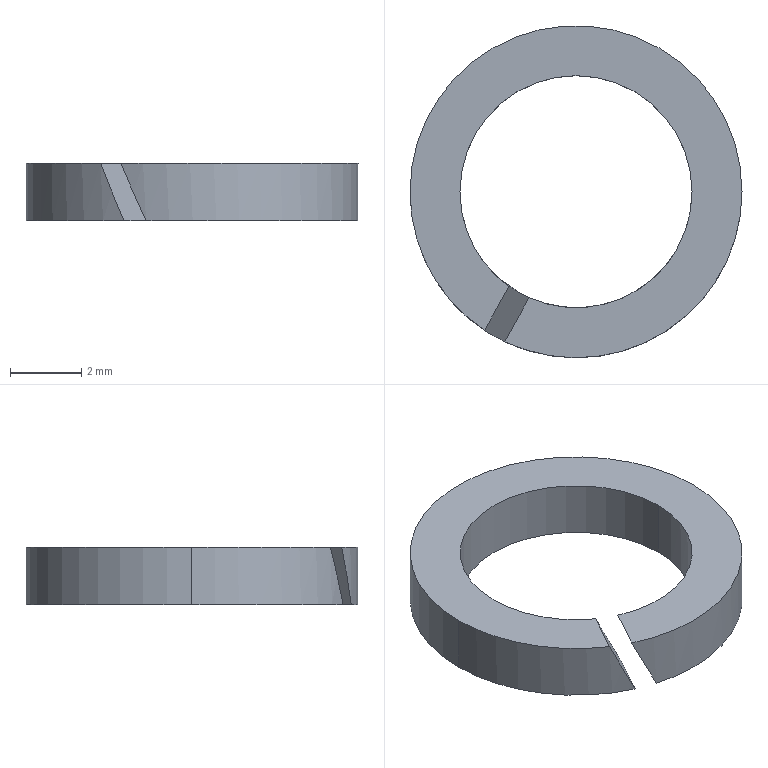Part | SolidWorks | features BaseBody 1 | 1 solid | 10 faces | box 9.3 x 9.3 x 1.6 mm | volume 54.128 mm3 | cylinder 6 | plane 4 | commonest cylinder face diameters 6.5 x3 9.3 x3
STEP:
#1=CARTESIAN_POINT('',(-40.153,-58.725,-65.029));
#2=VERTEX_POINT('',#1);
#3=CARTESIAN_POINT('',(-44.719,-61.697,-65.029));
#4=VERTEX_POINT('',#3);
#5=CARTESIAN_POINT('',(-43.403,-58.725,-65.029));
#6=DIRECTION('',(-0.000001053,0.,-1.));
#7=DIRECTION('',(-1.,0.,0.000001053));
#8=AXIS2_PLACEMENT_3D('',#5,#6,#7);
#9=CIRCLE('',#8,3.25);
#10=EDGE_CURVE('',#2,#4,#9,.T.);
#11=ORIENTED_EDGE('',*,*,#10,.F.);
#12=CARTESIAN_POINT('',(-40.153,-58.725,-66.629));
#13=VERTEX_POINT('',#12);
#14=CARTESIAN_POINT('',(-40.153,-58.725,-65.029));
#15=DIRECTION('',(-0.000001053,0.,-1.));
#16=VECTOR('',#15,1000.);
#17=LINE('',#14,#16);
#18=EDGE_CURVE('',#2,#13,#17,.T.);
#19=ORIENTED_EDGE('',*,*,#18,.T.);
#20=CARTESIAN_POINT('',(-43.991,-61.921,-66.629));
#21=VERTEX_POINT('',#20);
#22=CARTESIAN_POINT('',(-43.403,-58.725,-66.629));
#23=DIRECTION('',(0.000001053,0.,1.));
#24=DIRECTION('',(-1.,0.,0.000001053));
#25=AXIS2_PLACEMENT_3D('',#22,#23,#24);
#26=CIRCLE('',#25,3.25);
#27=EDGE_CURVE('',#21,#13,#26,.T.);
#28=ORIENTED_EDGE('',*,*,#27,.F.);
#29=CARTESIAN_POINT('',(-44.719,-61.697,-65.029));
#30=CARTESIAN_POINT('',(-44.486,-61.8,-65.574));
#31=CARTESIAN_POINT('',(-44.242,-61.875,-66.11));
#32=CARTESIAN_POINT('',(-43.991,-61.921,-66.629));
#33=(BOUNDED_CURVE()B_SPLINE_CURVE(3,(#29,#30,#31,#32),.UNSPECIFIED.,.F.,.T.)B_SPLINE_CURVE_WITH_KNOTS((4,4),(4.8,5.035),.UNSPECIFIED.)CURVE()GEOMETRIC_REPRESENTATION_ITEM()RATIONAL_B_SPLINE_CURVE((1.,0.9954,0.9954,1.))REPRESENTATION_ITEM(''));
#34=EDGE_CURVE('',#4,#21,#33,.T.);
#35=ORIENTED_EDGE('',*,*,#34,.F.);
#36=EDGE_LOOP('',(#11,#19,#28,#35));
#37=FACE_OUTER_BOUND('',#36,.T.);
#38=CARTESIAN_POINT('',(-43.403,-58.725,-65.029));
#39=DIRECTION('',(-0.000001053,0.,-1.));
#40=DIRECTION('',(-1.,0.,0.000001053));
#41=AXIS2_PLACEMENT_3D('',#38,#39,#40);
#42=CYLINDRICAL_SURFACE('',#41,3.25);
#43=ADVANCED_FACE('',(#37),#42,.F.);
#44=ORIENTED_EDGE('',*,*,#18,.F.);
#45=CARTESIAN_POINT('',(-46.653,-58.725,-65.029));
#46=VERTEX_POINT('',#45);
#47=CARTESIAN_POINT('',(-43.403,-58.725,-65.029));
#48=DIRECTION('',(-0.000001053,0.,-1.));
#49=DIRECTION('',(-1.,0.,0.000001053));
#50=AXIS2_PLACEMENT_3D('',#47,#48,#49);
#51=CIRCLE('',#50,3.25);
#52=EDGE_CURVE('',#46,#2,#51,.T.);
#53=ORIENTED_EDGE('',*,*,#52,.F.);
#54=CARTESIAN_POINT('',(-46.653,-58.725,-66.629));
#55=VERTEX_POINT('',#54);
#56=CARTESIAN_POINT('',(-46.653,-58.725,-65.029));
#57=DIRECTION('',(-0.000001053,0.,-1.));
#58=VECTOR('',#57,1000.);
#59=LINE('',#56,#58);
#60=EDGE_CURVE('',#46,#55,#59,.T.);
#61=ORIENTED_EDGE('',*,*,#60,.T.);
#62=CARTESIAN_POINT('',(-43.403,-58.725,-66.629));
#63=DIRECTION('',(0.000001053,0.,1.));
#64=DIRECTION('',(-1.,0.,0.000001053));
#65=AXIS2_PLACEMENT_3D('',#62,#63,#64);
#66=CIRCLE('',#65,3.25);
#67=EDGE_CURVE('',#13,#55,#66,.T.);
#68=ORIENTED_EDGE('',*,*,#67,.F.);
#69=EDGE_LOOP('',(#44,#53,#61,#68));
#70=FACE_OUTER_BOUND('',#69,.T.);
#71=CARTESIAN_POINT('',(-43.403,-58.725,-65.029));
#72=DIRECTION('',(-0.000001053,0.,-1.));
#73=DIRECTION('',(-1.,0.,0.000001053));
#74=AXIS2_PLACEMENT_3D('',#71,#72,#73);
#75=CYLINDRICAL_SURFACE('',#74,3.25);
#76=ADVANCED_FACE('',(#70),#75,.F.);
#77=CARTESIAN_POINT('',(-38.753,-58.725,-65.029));
#78=VERTEX_POINT('',#77);
#79=CARTESIAN_POINT('',(-48.053,-58.725,-65.029));
#80=VERTEX_POINT('',#79);
#81=CARTESIAN_POINT('',(-43.403,-58.725,-65.029));
#82=DIRECTION('',(0.000001053,0.,1.));
#83=DIRECTION('',(-1.,0.,0.000001053));
#84=AXIS2_PLACEMENT_3D('',#81,#82,#83);
#85=CIRCLE('',#84,4.65);
#86=EDGE_CURVE('',#78,#80,#85,.T.);
#87=ORIENTED_EDGE('',*,*,#86,.F.);
#88=CARTESIAN_POINT('',(-38.753,-58.725,-66.629));
#89=VERTEX_POINT('',#88);
#90=CARTESIAN_POINT('',(-38.753,-58.725,-65.029));
#91=DIRECTION('',(-0.000001053,0.,-1.));
#92=VECTOR('',#91,1000.);
#93=LINE('',#90,#92);
#94=EDGE_CURVE('',#78,#89,#93,.T.);
#95=ORIENTED_EDGE('',*,*,#94,.T.);
#96=CARTESIAN_POINT('',(-48.053,-58.725,-66.629));
#97=VERTEX_POINT('',#96);
#98=CARTESIAN_POINT('',(-43.403,-58.725,-66.629));
#99=DIRECTION('',(0.000001053,0.,1.));
#100=DIRECTION('',(-1.,0.,0.000001053));
#101=AXIS2_PLACEMENT_3D('',#98,#99,#100);
#102=CIRCLE('',#101,4.65);
#103=EDGE_CURVE('',#89,#97,#102,.T.);
#104=ORIENTED_EDGE('',*,*,#103,.T.);
#105=CARTESIAN_POINT('',(-48.053,-58.725,-65.029));
#106=DIRECTION('',(-0.000001053,0.,-1.));
#107=VECTOR('',#106,1000.);
#108=LINE('',#105,#107);
#109=EDGE_CURVE('',#80,#97,#108,.T.);
#110=ORIENTED_EDGE('',*,*,#109,.F.);
#111=EDGE_LOOP('',(#87,#95,#104,#110));
#112=FACE_OUTER_BOUND('',#111,.T.);
#113=CARTESIAN_POINT('',(-43.403,-58.725,-65.029));
#114=DIRECTION('',(-0.000001053,0.,-1.));
#115=DIRECTION('',(-1.,0.,0.000001053));
#116=AXIS2_PLACEMENT_3D('',#113,#114,#115);
#117=CYLINDRICAL_SURFACE('',#116,4.65);
#118=ADVANCED_FACE('',(#112),#117,.T.);
#119=CARTESIAN_POINT('',(-45.964,-62.607,-65.029));
#120=VERTEX_POINT('',#119);
#121=CARTESIAN_POINT('',(-43.403,-58.725,-65.029));
#122=DIRECTION('',(0.000001053,0.,1.));
#123=DIRECTION('',(-1.,0.,0.000001053));
#124=AXIS2_PLACEMENT_3D('',#121,#122,#123);
#125=CIRCLE('',#124,4.65);
#126=EDGE_CURVE('',#80,#120,#125,.T.);
#127=ORIENTED_EDGE('',*,*,#126,.F.);
#128=ORIENTED_EDGE('',*,*,#109,.T.);
#129=CARTESIAN_POINT('',(-45.31,-62.966,-66.629));
#130=VERTEX_POINT('',#129);
#131=CARTESIAN_POINT('',(-43.403,-58.725,-66.629));
#132=DIRECTION('',(0.000001053,0.,1.));
#133=DIRECTION('',(-1.,0.,0.000001053));
#134=AXIS2_PLACEMENT_3D('',#131,#132,#133);
#135=CIRCLE('',#134,4.65);
#136=EDGE_CURVE('',#97,#130,#135,.T.);
#137=ORIENTED_EDGE('',*,*,#136,.T.);
#138=CARTESIAN_POINT('',(-45.31,-62.966,-66.629));
#139=CARTESIAN_POINT('',(-45.537,-62.864,-66.096));
#140=CARTESIAN_POINT('',(-45.756,-62.744,-65.562));
#141=CARTESIAN_POINT('',(-45.964,-62.607,-65.029));
#142=(BOUNDED_CURVE()B_SPLINE_CURVE(3,(#138,#139,#140,#141),.UNSPECIFIED.,.F.,.F.)B_SPLINE_CURVE_WITH_KNOTS((4,4),(1.489,1.65),.UNSPECIFIED.)CURVE()GEOMETRIC_REPRESENTATION_ITEM()RATIONAL_B_SPLINE_CURVE((1.,0.9979,0.9979,1.))REPRESENTATION_ITEM(''));
#143=EDGE_CURVE('',#130,#120,#142,.T.);
#144=ORIENTED_EDGE('',*,*,#143,.T.);
#145=EDGE_LOOP('',(#127,#128,#137,#144));
#146=FACE_OUTER_BOUND('',#145,.T.);
#147=CARTESIAN_POINT('',(-43.403,-58.725,-65.029));
#148=DIRECTION('',(-0.000001053,0.,-1.));
#149=DIRECTION('',(-1.,0.,0.000001053));
#150=AXIS2_PLACEMENT_3D('',#147,#148,#149);
#151=CYLINDRICAL_SURFACE('',#150,4.65);
#152=ADVANCED_FACE('',(#146),#151,.T.);
#153=CARTESIAN_POINT('',(-45.284,-61.375,-65.029));
#154=VERTEX_POINT('',#153);
#155=CARTESIAN_POINT('',(-45.627,-61.997,-65.029));
#156=DIRECTION('',(-0.483,-0.8756,0.));
#157=VECTOR('',#156,1000.);
#158=LINE('',#155,#157);
#159=EDGE_CURVE('',#154,#120,#158,.T.);
#160=ORIENTED_EDGE('',*,*,#159,.F.);
#161=CARTESIAN_POINT('',(-43.403,-58.725,-65.029));
#162=DIRECTION('',(-0.000001053,0.,-1.));
#163=DIRECTION('',(-1.,0.,0.000001053));
#164=AXIS2_PLACEMENT_3D('',#161,#162,#163);
#165=CIRCLE('',#164,3.25);
#166=EDGE_CURVE('',#154,#46,#165,.T.);
#167=ORIENTED_EDGE('',*,*,#166,.T.);
#168=ORIENTED_EDGE('',*,*,#52,.T.);
#169=ORIENTED_EDGE('',*,*,#10,.T.);
#170=CARTESIAN_POINT('',(-45.397,-62.926,-65.029));
#171=VERTEX_POINT('',#170);
#172=CARTESIAN_POINT('',(-45.021,-62.243,-65.029));
#173=DIRECTION('',(-0.483,-0.8756,0.));
#174=VECTOR('',#173,1000.);
#175=LINE('',#172,#174);
#176=EDGE_CURVE('',#4,#171,#175,.T.);
#177=ORIENTED_EDGE('',*,*,#176,.T.);
#178=CARTESIAN_POINT('',(-43.403,-58.725,-65.029));
#179=DIRECTION('',(0.000001053,0.,1.));
#180=DIRECTION('',(-1.,0.,0.000001053));
#181=AXIS2_PLACEMENT_3D('',#178,#179,#180);
#182=CIRCLE('',#181,4.65);
#183=EDGE_CURVE('',#171,#78,#182,.T.);
#184=ORIENTED_EDGE('',*,*,#183,.T.);
#185=ORIENTED_EDGE('',*,*,#86,.T.);
#186=ORIENTED_EDGE('',*,*,#126,.T.);
#187=EDGE_LOOP('',(#160,#167,#168,#169,#177,#184,#185,#186));
#188=FACE_OUTER_BOUND('',#187,.T.);
#189=CARTESIAN_POINT('',(-43.403,-58.725,-65.029));
#190=DIRECTION('',(0.000001053,0.,1.));
#191=DIRECTION('',(1.,0.,-0.000001053));
#192=AXIS2_PLACEMENT_3D('',#189,#190,#191);
#193=PLANE('',#192);
#194=ADVANCED_FACE('',(#188),#193,.T.);
#195=ORIENTED_EDGE('',*,*,#60,.F.);
#196=ORIENTED_EDGE('',*,*,#166,.F.);
#197=CARTESIAN_POINT('',(-44.63,-61.735,-66.629));
#198=VERTEX_POINT('',#197);
#199=CARTESIAN_POINT('',(-44.63,-61.735,-66.629));
#200=CARTESIAN_POINT('',(-44.862,-61.64,-66.097));
#201=CARTESIAN_POINT('',(-45.081,-61.52,-65.561));
#202=CARTESIAN_POINT('',(-45.284,-61.375,-65.029));
#203=(BOUNDED_CURVE()B_SPLINE_CURVE(3,(#199,#200,#201,#202),.UNSPECIFIED.,.F.,.F.)B_SPLINE_CURVE_WITH_KNOTS((4,4),(1.454,1.684),.UNSPECIFIED.)CURVE()GEOMETRIC_REPRESENTATION_ITEM()RATIONAL_B_SPLINE_CURVE((1.,0.9956,0.9956,1.))REPRESENTATION_ITEM(''));
#204=EDGE_CURVE('',#198,#154,#203,.T.);
#205=ORIENTED_EDGE('',*,*,#204,.F.);
#206=CARTESIAN_POINT('',(-43.403,-58.725,-66.629));
#207=DIRECTION('',(0.000001053,0.,1.));
#208=DIRECTION('',(-1.,0.,0.000001053));
#209=AXIS2_PLACEMENT_3D('',#206,#207,#208);
#210=CIRCLE('',#209,3.25);
#211=EDGE_CURVE('',#55,#198,#210,.T.);
#212=ORIENTED_EDGE('',*,*,#211,.F.);
#213=EDGE_LOOP('',(#195,#196,#205,#212));
#214=FACE_OUTER_BOUND('',#213,.T.);
#215=CARTESIAN_POINT('',(-43.403,-58.725,-65.029));
#216=DIRECTION('',(-0.000001053,0.,-1.));
#217=DIRECTION('',(-1.,0.,0.000001053));
#218=AXIS2_PLACEMENT_3D('',#215,#216,#217);
#219=CYLINDRICAL_SURFACE('',#218,3.25);
#220=ADVANCED_FACE('',(#214),#219,.F.);
#221=ORIENTED_EDGE('',*,*,#94,.F.);
#222=ORIENTED_EDGE('',*,*,#183,.F.);
#223=CARTESIAN_POINT('',(-44.693,-63.193,-66.629));
#224=VERTEX_POINT('',#223);
#225=CARTESIAN_POINT('',(-45.397,-62.926,-65.029));
#226=CARTESIAN_POINT('',(-45.17,-63.034,-65.568));
#227=CARTESIAN_POINT('',(-44.934,-63.123,-66.103));
#228=CARTESIAN_POINT('',(-44.693,-63.193,-66.629));
#229=(BOUNDED_CURVE()B_SPLINE_CURVE(3,(#225,#226,#227,#228),.UNSPECIFIED.,.F.,.T.)B_SPLINE_CURVE_WITH_KNOTS((4,4),(4.773,4.936),.UNSPECIFIED.)CURVE()GEOMETRIC_REPRESENTATION_ITEM()RATIONAL_B_SPLINE_CURVE((1.,0.9978,0.9978,1.))REPRESENTATION_ITEM(''));
#230=EDGE_CURVE('',#171,#224,#229,.T.);
#231=ORIENTED_EDGE('',*,*,#230,.T.);
#232=CARTESIAN_POINT('',(-43.403,-58.725,-66.629));
#233=DIRECTION('',(0.000001053,0.,1.));
#234=DIRECTION('',(-1.,0.,0.000001053));
#235=AXIS2_PLACEMENT_3D('',#232,#233,#234);
#236=CIRCLE('',#235,4.65);
#237=EDGE_CURVE('',#224,#89,#236,.T.);
#238=ORIENTED_EDGE('',*,*,#237,.T.);
#239=EDGE_LOOP('',(#221,#222,#231,#238));
#240=FACE_OUTER_BOUND('',#239,.T.);
#241=CARTESIAN_POINT('',(-43.403,-58.725,-65.029));
#242=DIRECTION('',(-0.000001053,0.,-1.));
#243=DIRECTION('',(-1.,0.,0.000001053));
#244=AXIS2_PLACEMENT_3D('',#241,#242,#243);
#245=CYLINDRICAL_SURFACE('',#244,4.65);
#246=ADVANCED_FACE('',(#240),#245,.T.);
#247=CARTESIAN_POINT('',(-44.974,-62.357,-66.629));
#248=DIRECTION('',(0.483,0.8756,0.));
#249=VECTOR('',#248,1000.);
#250=LINE('',#247,#249);
#251=EDGE_CURVE('',#130,#198,#250,.T.);
#252=ORIENTED_EDGE('',*,*,#251,.T.);
#253=ORIENTED_EDGE('',*,*,#204,.T.);
#254=ORIENTED_EDGE('',*,*,#159,.T.);
#255=ORIENTED_EDGE('',*,*,#143,.F.);
#256=EDGE_LOOP('',(#252,#253,#254,#255));
#257=FACE_OUTER_BOUND('',#256,.T.);
#258=CARTESIAN_POINT('',(-45.301,-62.177,-65.829));
#259=DIRECTION('',(0.7936,-0.4378,0.4226));
#260=DIRECTION('',(0.483,0.8756,0.));
#261=AXIS2_PLACEMENT_3D('',#258,#259,#260);
#262=PLANE('',#261);
#263=ADVANCED_FACE('',(#257),#262,.T.);
#264=ORIENTED_EDGE('',*,*,#251,.F.);
#265=ORIENTED_EDGE('',*,*,#136,.F.);
#266=ORIENTED_EDGE('',*,*,#103,.F.);
#267=ORIENTED_EDGE('',*,*,#237,.F.);
#268=CARTESIAN_POINT('',(-43.991,-61.921,-66.629));
#269=DIRECTION('',(-0.483,-0.8756,0.000000509));
#270=VECTOR('',#269,1000.);
#271=LINE('',#268,#270);
#272=EDGE_CURVE('',#21,#224,#271,.T.);
#273=ORIENTED_EDGE('',*,*,#272,.F.);
#274=ORIENTED_EDGE('',*,*,#27,.T.);
#275=ORIENTED_EDGE('',*,*,#67,.T.);
#276=ORIENTED_EDGE('',*,*,#211,.T.);
#277=EDGE_LOOP('',(#264,#265,#266,#267,#273,#274,#275,#276));
#278=FACE_OUTER_BOUND('',#277,.T.);
#279=CARTESIAN_POINT('',(-43.403,-58.725,-66.629));
#280=DIRECTION('',(0.000001053,0.,1.));
#281=DIRECTION('',(1.,0.,-0.000001053));
#282=AXIS2_PLACEMENT_3D('',#279,#280,#281);
#283=PLANE('',#282);
#284=ADVANCED_FACE('',(#278),#283,.F.);
#285=ORIENTED_EDGE('',*,*,#176,.F.);
#286=ORIENTED_EDGE('',*,*,#34,.T.);
#287=ORIENTED_EDGE('',*,*,#272,.T.);
#288=ORIENTED_EDGE('',*,*,#230,.F.);
#289=EDGE_LOOP('',(#285,#286,#287,#288));
#290=FACE_OUTER_BOUND('',#289,.T.);
#291=CARTESIAN_POINT('',(-44.694,-62.424,-65.829));
#292=DIRECTION('',(0.7936,-0.4378,0.4226));
#293=DIRECTION('',(0.483,0.8756,0.));
#294=AXIS2_PLACEMENT_3D('',#291,#292,#293);
#295=PLANE('',#294);
#296=ADVANCED_FACE('',(#290),#295,.F.);
#297=CLOSED_SHELL('',(#43,#76,#118,#152,#194,#220,#246,#263,#284,#296));
#298=MANIFOLD_SOLID_BREP('',#297);
#299=CARTESIAN_POINT('',(0.,0.,0.));
#300=DIRECTION('',(0.,0.,1.));
#301=DIRECTION('',(1.,0.,0.));
#302=AXIS2_PLACEMENT_3D('',#299,#300,#301);
#303=(LENGTH_UNIT()NAMED_UNIT(*)SI_UNIT(.MILLI.,.METRE.));
#304=UNCERTAINTY_MEASURE_WITH_UNIT(LENGTH_MEASURE(0.00001),#303,'','');
#305=(NAMED_UNIT(*)PLANE_ANGLE_UNIT()SI_UNIT($,.RADIAN.));
#306=(NAMED_UNIT(*)SI_UNIT($,.STERADIAN.)SOLID_ANGLE_UNIT());
#307=(GEOMETRIC_REPRESENTATION_CONTEXT(3)GLOBAL_UNCERTAINTY_ASSIGNED_CONTEXT((#304))GLOBAL_UNIT_ASSIGNED_CONTEXT((#303,#305,#306))REPRESENTATION_CONTEXT('',''));
#308=ADVANCED_BREP_SHAPE_REPRESENTATION('',(#298,#302),#307);